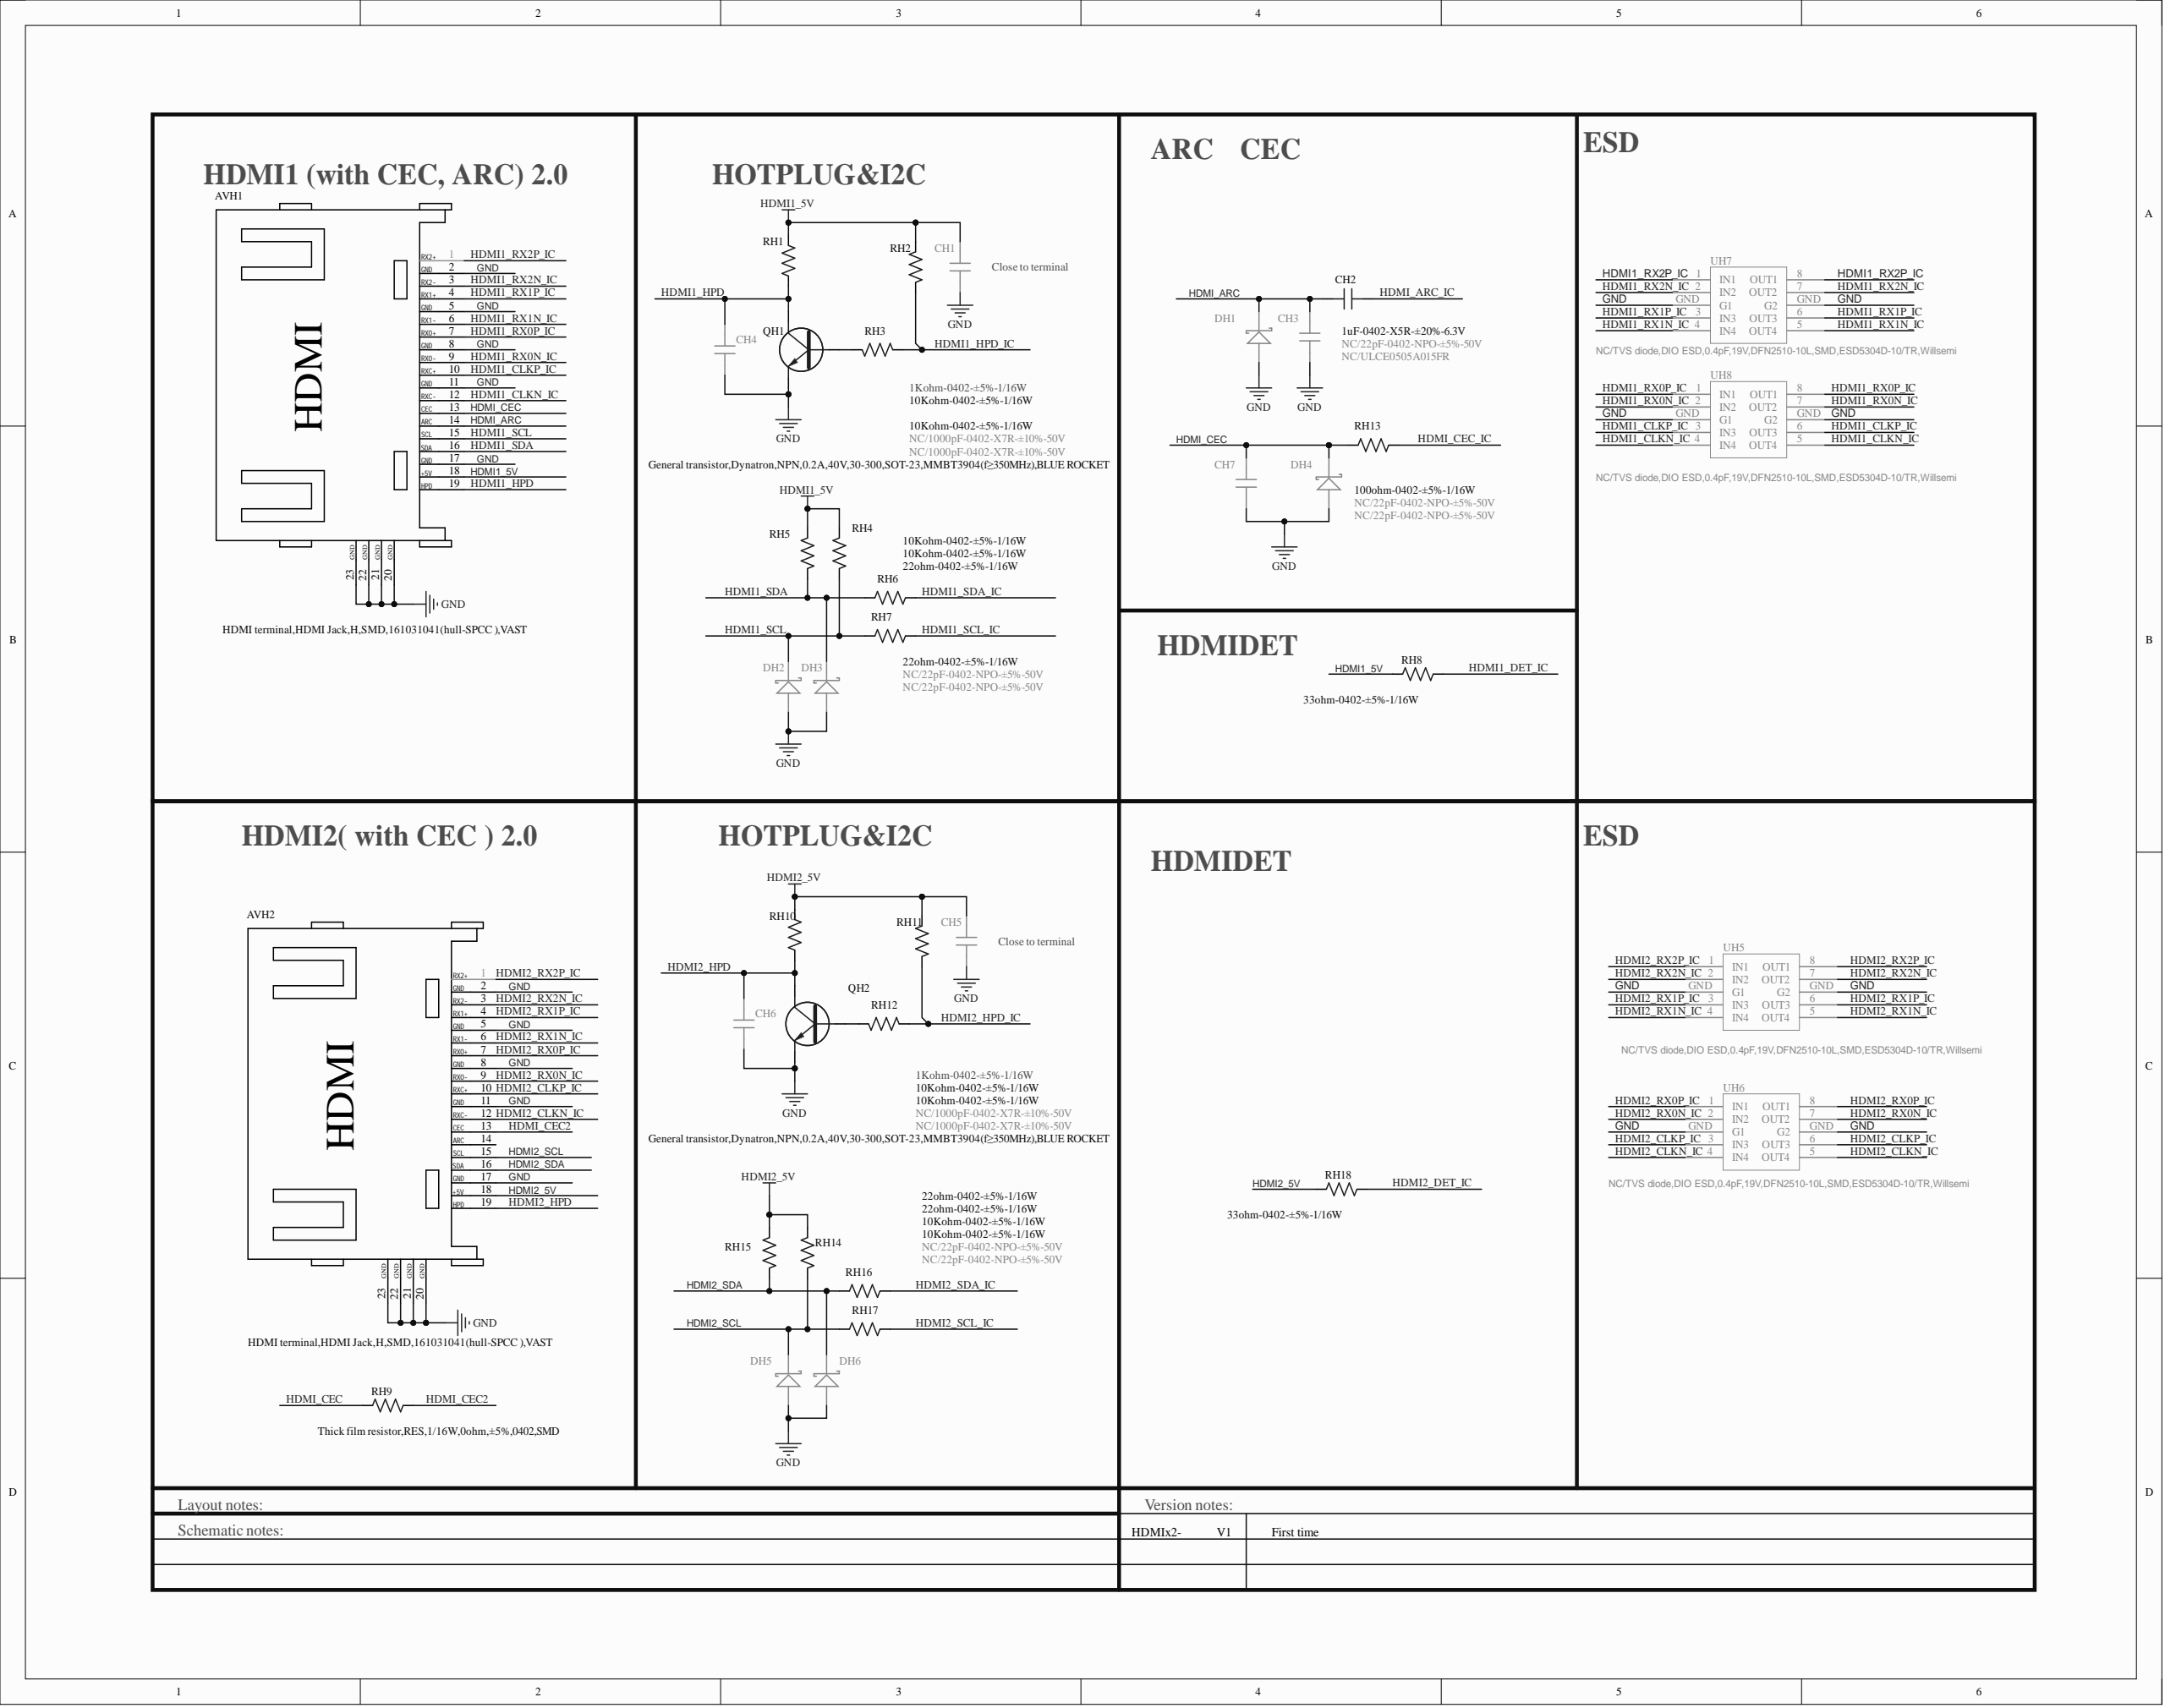Circuit board | Altium Designer | 951 parts | 509 nets | one sheet of the schematic
Parts on this sheet (reference | value | footprint):
AVH1 | HDMI terminal,HDMI Jack,H,SMD,161031041(hull-SPCC ),VAST | HDMI-HS-1
AVH2 | HDMI terminal,HDMI Jack,H,SMD,161031041(hull-SPCC ),VAST | HDMI-HS-1
CH1 | NC/1000pF-0402-X7R-±10%-50V | C0402
CH2 | 1uF-0402-X5R-±20%-6.3V | C0402
CH3 | NC/22pF-0402-NPO-±5%-50V | C0402
CH4 | NC/1000pF-0402-X7R-±10%-50V | C0402
CH5 | NC/1000pF-0402-X7R-±10%-50V | C0402
CH6 | NC/1000pF-0402-X7R-±10%-50V | C0402
CH7 | NC/22pF-0402-NPO-±5%-50V | C0402
DH1 | NC/ULCE0505A015FR | DIODE-S0402
DH2 | NC/22pF-0402-NPO-±5%-50V | DIODE-S0402
DH3 | NC/22pF-0402-NPO-±5%-50V | DIODE-S0402
DH4 | NC/22pF-0402-NPO-±5%-50V | DIODE-S0402
DH5 | NC/22pF-0402-NPO-±5%-50V | DIODE-S0402
DH6 | NC/22pF-0402-NPO-±5%-50V | DIODE-S0402
QH1 | General transistor,Dynatron,NPN,0.2A,40V,30-300,SOT-23,MMBT3904(f=350MHz),BLUE ROCKET | SOT-23
QH2 | General transistor,Dynatron,NPN,0.2A,40V,30-300,SOT-23,MMBT3904(f=350MHz),BLUE ROCKET | SOT-23
RH1 | 1Kohm-0402-±5%-1/16W | R0402
RH2 | 10Kohm-0402-±5%-1/16W | R0402
RH3 | 10Kohm-0402-±5%-1/16W | R0402
RH4 | 10Kohm-0402-±5%-1/16W | R0402
RH5 | 10Kohm-0402-±5%-1/16W | R0402
RH6 | 22ohm-0402-±5%-1/16W | R0402
RH7 | 22ohm-0402-±5%-1/16W | R0402
RH8 | 33ohm-0402-±5%-1/16W | R0402
RH9 | Thick film resistor,RES,1/16W,0ohm,±5%,0402,SMD | R0402
RH10 | 1Kohm-0402-±5%-1/16W | R0402
RH11 | 10Kohm-0402-±5%-1/16W | R0402
RH12 | 10Kohm-0402-±5%-1/16W | R0402
RH13 | 100ohm-0402-±5%-1/16W | R0402
RH14 | 10Kohm-0402-±5%-1/16W | R0402
RH15 | 10Kohm-0402-±5%-1/16W | R0402
RH16 | 22ohm-0402-±5%-1/16W | R0402
RH17 | 22ohm-0402-±5%-1/16W | R0402
RH18 | 33ohm-0402-±5%-1/16W | R0402
UH5 | NC/TVS diode,DIO ESD,0.4pF,19V,DFN2510-10L,SMD,ESD5304D-10/TR,Willsemi | RCL0524P
UH6 | NC/TVS diode,DIO ESD,0.4pF,19V,DFN2510-10L,SMD,ESD5304D-10/TR,Willsemi | RCL0524P
UH7 | NC/TVS diode,DIO ESD,0.4pF,19V,DFN2510-10L,SMD,ESD5304D-10/TR,Willsemi | RCL0524P
UH8 | NC/TVS diode,DIO ESD,0.4pF,19V,DFN2510-10L,SMD,ESD5304D-10/TR,Willsemi | RCL0524P
Nets of these parts (net: part-pin ...):
NetQH2_B: QH2-B RH12-1
NetQH1_B: QH1-B RH3-1
HDMI_CEC_IC: RH13-2
HDMI_CEC2: RH9-1 AVH2-13
HDMI_CEC: CH7-2 DH4-K RH9-2 RH13-1 AVH1-13
HDMI_ARC_IC: CH2-2
HDMI_ARC: CH2-1 CH3-2 DH1-K AVH1-14
HDMI2_SDA_IC: RH16-2
HDMI2_SDA: DH6-K RH15-2 RH16-1 AVH2-16
HDMI2_SCL_IC: RH17-2
HDMI2_SCL: DH5-K RH14-2 RH17-1 AVH2-15
HDMI2_RX2P_IC: UH5-1 UH5-8 AVH2-1
HDMI2_RX2N_IC: UH5-2 UH5-7 AVH2-3
HDMI2_RX1P_IC: UH5-3 UH5-6 AVH2-4
HDMI2_RX1N_IC: UH5-4 UH5-5 AVH2-6
HDMI2_RX0P_IC: UH6-1 UH6-8 AVH2-7
HDMI2_RX0N_IC: UH6-2 UH6-7 AVH2-9
HDMI2_HPD_IC: RH11-2 RH12-2
HDMI2_HPD: CH6-2 QH2-C RH10-2 AVH2-19
HDMI2_DET_IC: RH18-2
HDMI2_CLKP_IC: UH6-3 UH6-6 AVH2-10
HDMI2_CLKN_IC: UH6-4 UH6-5 AVH2-12
HDMI2_5V: CH5-1 RH10-1 RH11-1 RH14-1 RH15-1 RH18-1 AVH2-18
HDMI1_SDA_IC: RH6-2
HDMI1_SDA: DH3-K RH5-2 RH6-1 AVH1-16
HDMI1_SCL_IC: RH7-2
HDMI1_SCL: DH2-K RH4-2 RH7-1 AVH1-15
HDMI1_RX2P_IC: UH7-1 UH7-8 AVH1-1
HDMI1_RX2N_IC: UH7-2 UH7-7 AVH1-3
HDMI1_RX1P_IC: UH7-3 UH7-6 AVH1-4
HDMI1_RX1N_IC: UH7-4 UH7-5 AVH1-6
HDMI1_RX0P_IC: UH8-1 UH8-8 AVH1-7
HDMI1_RX0N_IC: UH8-2 UH8-7 AVH1-9
HDMI1_HPD_IC: RH2-2 RH3-2
HDMI1_HPD: CH4-2 QH1-C RH1-2 AVH1-19
HDMI1_DET_IC: RH8-2
HDMI1_CLKP_IC: UH8-3 UH8-6 AVH1-10
HDMI1_CLKN_IC: UH8-4 UH8-5 AVH1-12
HDMI1_5V: CH1-1 RH1-1 RH2-1 RH4-1 RH5-1 RH8-1 AVH1-18
GND: CH1-2 CH3-1 CH4-1 CH5-2 CH6-1 CH7-1 DH1-A DH2-A DH3-A DH4-A DH5-A DH6-A QH1-E QH2-E UH5-GND UH6-GND UH7-GND UH8-GND AVH1-2 AVH1-5 AVH1-8 AVH1-11 AVH1-17 AVH1-20 AVH1-21 AVH1-22 AVH1-23 AVH2-2 AVH2-5 AVH2-8 AVH2-11 AVH2-17 AVH2-20 AVH2-21 AVH2-22 AVH2-23